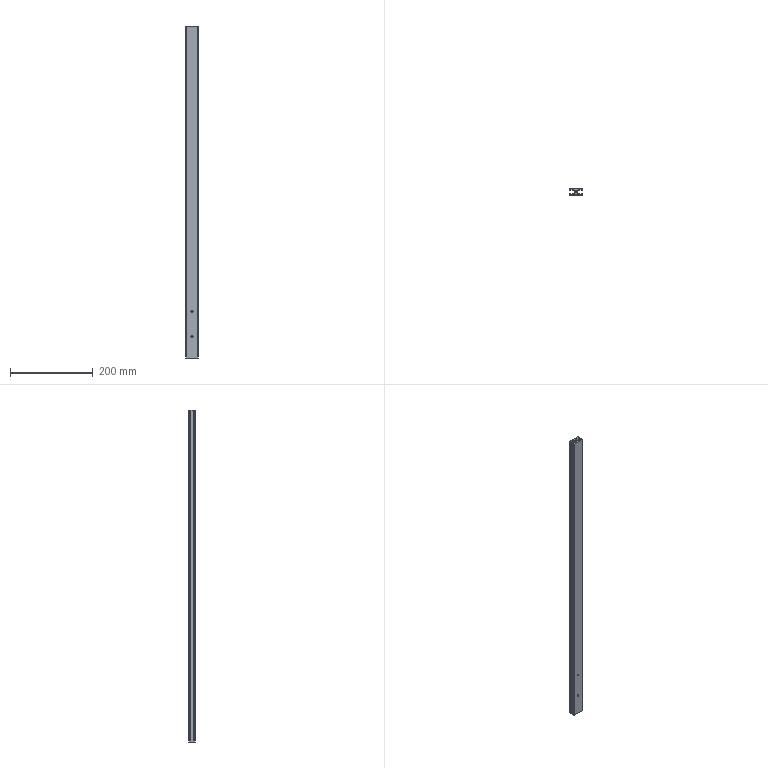Part | SolidWorks | features BaseBody 1, HoleWzd 1, MoveFace 1 | 1 solid | 87 faces | box 30 x 15 x 802 mm | volume 193016 mm3 | plane 46 | cylinder 41 | commonest cylinder face diameters 5 x31 1 x6 2 x4